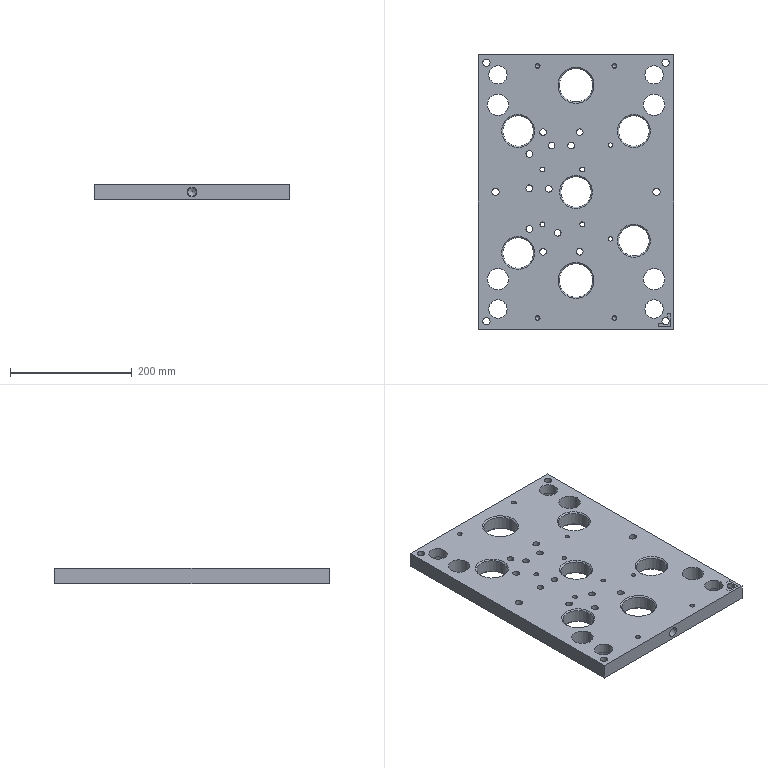Part | STEP file | DZMB | 1 solid | 138 faces | box 320 x 450 x 25 mm | volume 2980315 mm3 | cylinder 74 | plane 44 | cone 20 | commonest cylinder face diameters 16 x14 11 x13 8 x10 12 x10 50 x5 6.7 x4